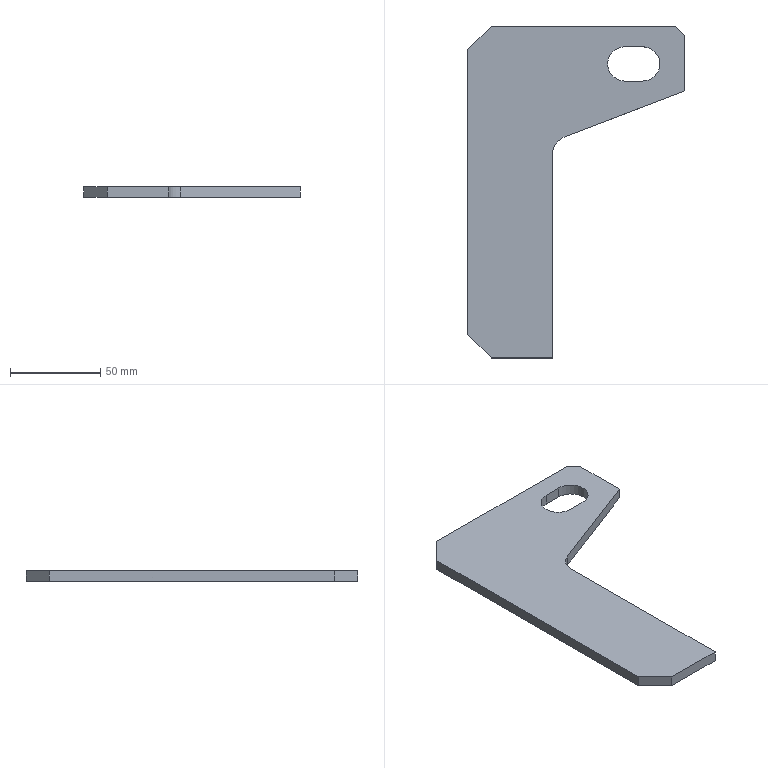Part | STEP file | 筋Plate-200×100-5 | 1 solid | 17 faces | box 120 x 184 x 6 mm | volume 69909 mm3 | plane 13 | cylinder 4 | commonest cylinder face diameters 19 x3 20 x1
STEP:
#1=CARTESIAN_POINT('',(0.,0.,0.));
#2=DIRECTION('',(0.,0.,1.));
#3=DIRECTION('',(1.,0.,0.));
#4=AXIS2_PLACEMENT_3D('',#1,#2,#3);
#5=CARTESIAN_POINT('',(27.,80.5,3.));
#6=VERTEX_POINT('',#5);
#7=CARTESIAN_POINT('',(27.,80.5,-3.));
#8=VERTEX_POINT('',#7);
#9=CARTESIAN_POINT('',(27.,80.5,-3.));
#10=DIRECTION('',(0.,0.,-1.));
#11=VECTOR('',#10,1.);
#12=LINE('',#9,#11);
#13=CARTESIAN_POINT('',(27.,71.,-3.));
#14=DIRECTION('',(0.,0.,-1.));
#15=DIRECTION('',(-1.,0.,0.));
#16=AXIS2_PLACEMENT_3D('',#13,#14,#15);
#17=CYLINDRICAL_SURFACE('',#16,9.5);
#18=CARTESIAN_POINT('',(1.571,0.));
#19=DIRECTION('',(0.,1.));
#20=VECTOR('',#19,1.);
#21=LINE('',#18,#20);
#22=(GEOMETRIC_REPRESENTATION_CONTEXT(2)PARAMETRIC_REPRESENTATION_CONTEXT()REPRESENTATION_CONTEXT('',''));
#23=DEFINITIONAL_REPRESENTATION('',(#21),#22);
#24=PCURVE('',#17,#23);
#25=CARTESIAN_POINT('',(37.,80.5,-3.));
#26=DIRECTION('',(0.,1.,0.));
#27=DIRECTION('',(0.,0.,1.));
#28=AXIS2_PLACEMENT_3D('',#25,#26,#27);
#29=PLANE('',#28);
#30=CARTESIAN_POINT('',(0.,-10.));
#31=DIRECTION('',(-1.,0.));
#32=VECTOR('',#31,1.);
#33=LINE('',#30,#32);
#34=(GEOMETRIC_REPRESENTATION_CONTEXT(2)PARAMETRIC_REPRESENTATION_CONTEXT()REPRESENTATION_CONTEXT('',''));
#35=DEFINITIONAL_REPRESENTATION('',(#33),#34);
#36=PCURVE('',#29,#35);
#37=SURFACE_CURVE('',#12,(#24,#36),.PCURVE_S1.);
#38=EDGE_CURVE('',#6,#8,#37,.T.);
#39=ORIENTED_EDGE('',*,*,#38,.T.);
#40=CARTESIAN_POINT('',(17.5,71.,-3.));
#41=VERTEX_POINT('',#40);
#42=CARTESIAN_POINT('',(27.,71.,-3.));
#43=DIRECTION('',(0.,0.,-1.));
#44=DIRECTION('',(-1.,0.,0.));
#45=AXIS2_PLACEMENT_3D('',#42,#43,#44);
#46=CIRCLE('',#45,9.5);
#47=CARTESIAN_POINT('',(0.,0.));
#48=DIRECTION('',(1.,0.));
#49=VECTOR('',#48,1.);
#50=LINE('',#47,#49);
#51=(GEOMETRIC_REPRESENTATION_CONTEXT(2)PARAMETRIC_REPRESENTATION_CONTEXT()REPRESENTATION_CONTEXT('',''));
#52=DEFINITIONAL_REPRESENTATION('',(#50),#51);
#53=PCURVE('',#17,#52);
#54=CARTESIAN_POINT('',(0.,0.,-3.));
#55=DIRECTION('',(0.,0.,1.));
#56=DIRECTION('',(1.,0.,0.));
#57=AXIS2_PLACEMENT_3D('',#54,#55,#56);
#58=PLANE('',#57);
#59=CARTESIAN_POINT('',(17.5,71.));
#60=CARTESIAN_POINT('',(17.5,87.454));
#61=CARTESIAN_POINT('',(31.75,79.227));
#62=CARTESIAN_POINT('',(46.,71.));
#63=CARTESIAN_POINT('',(31.75,62.773));
#64=CARTESIAN_POINT('',(17.5,54.546));
#65=CARTESIAN_POINT('',(17.5,71.));
#66=(BOUNDED_CURVE()B_SPLINE_CURVE(2,(#59,#60,#61,#62,#63,#64,#65),.UNSPECIFIED.,.T.,.F.)B_SPLINE_CURVE_WITH_KNOTS((1,2,2,2,2,1),(-2.094,0.,2.094,4.189,6.283,8.378),.UNSPECIFIED.)CURVE()GEOMETRIC_REPRESENTATION_ITEM()RATIONAL_B_SPLINE_CURVE((1.,0.5,1.,0.5,1.,0.5,1.))REPRESENTATION_ITEM(''));
#67=(GEOMETRIC_REPRESENTATION_CONTEXT(2)PARAMETRIC_REPRESENTATION_CONTEXT()REPRESENTATION_CONTEXT('',''));
#68=DEFINITIONAL_REPRESENTATION('',(#66),#67);
#69=PCURVE('',#58,#68);
#70=SURFACE_CURVE('',#46,(#53,#69),.PCURVE_S1.);
#71=EDGE_CURVE('',#41,#8,#70,.T.);
#72=ORIENTED_EDGE('',*,*,#71,.F.);
#73=CARTESIAN_POINT('',(17.5,71.,3.));
#74=VERTEX_POINT('',#73);
#75=CARTESIAN_POINT('',(17.5,71.,-3.));
#76=DIRECTION('',(0.,0.,-1.));
#77=VECTOR('',#76,1.);
#78=LINE('',#75,#77);
#79=CARTESIAN_POINT('',(0.,0.));
#80=DIRECTION('',(0.,1.));
#81=VECTOR('',#80,1.);
#82=LINE('',#79,#81);
#83=(GEOMETRIC_REPRESENTATION_CONTEXT(2)PARAMETRIC_REPRESENTATION_CONTEXT()REPRESENTATION_CONTEXT('',''));
#84=DEFINITIONAL_REPRESENTATION('',(#82),#83);
#85=PCURVE('',#17,#84);
#86=CARTESIAN_POINT('',(27.,71.,-3.));
#87=DIRECTION('',(0.,0.,-1.));
#88=DIRECTION('',(-1.,0.,0.));
#89=AXIS2_PLACEMENT_3D('',#86,#87,#88);
#90=CYLINDRICAL_SURFACE('',#89,9.5);
#91=CARTESIAN_POINT('',(6.283,0.));
#92=DIRECTION('',(0.,1.));
#93=VECTOR('',#92,1.);
#94=LINE('',#91,#93);
#95=(GEOMETRIC_REPRESENTATION_CONTEXT(2)PARAMETRIC_REPRESENTATION_CONTEXT()REPRESENTATION_CONTEXT('',''));
#96=DEFINITIONAL_REPRESENTATION('',(#94),#95);
#97=PCURVE('',#90,#96);
#98=SURFACE_CURVE('',#78,(#85,#97),.PCURVE_S1.);
#99=EDGE_CURVE('',#74,#41,#98,.T.);
#100=ORIENTED_EDGE('',*,*,#99,.F.);
#101=CARTESIAN_POINT('',(27.,71.,3.));
#102=DIRECTION('',(0.,0.,1.));
#103=DIRECTION('',(1.,0.,0.));
#104=AXIS2_PLACEMENT_3D('',#101,#102,#103);
#105=CIRCLE('',#104,9.5);
#106=CARTESIAN_POINT('',(3.142,-6.));
#107=DIRECTION('',(-1.,0.));
#108=VECTOR('',#107,1.);
#109=LINE('',#106,#108);
#110=(GEOMETRIC_REPRESENTATION_CONTEXT(2)PARAMETRIC_REPRESENTATION_CONTEXT()REPRESENTATION_CONTEXT('',''));
#111=DEFINITIONAL_REPRESENTATION('',(#109),#110);
#112=PCURVE('',#17,#111);
#113=CARTESIAN_POINT('',(0.,0.,3.));
#114=DIRECTION('',(0.,0.,1.));
#115=DIRECTION('',(1.,0.,0.));
#116=AXIS2_PLACEMENT_3D('',#113,#114,#115);
#117=PLANE('',#116);
#118=CARTESIAN_POINT('',(27.,71.));
#119=DIRECTION('',(1.,0.));
#120=AXIS2_PLACEMENT_2D('',#118,#119);
#121=CIRCLE('',#120,9.5);
#122=(GEOMETRIC_REPRESENTATION_CONTEXT(2)PARAMETRIC_REPRESENTATION_CONTEXT()REPRESENTATION_CONTEXT('',''));
#123=DEFINITIONAL_REPRESENTATION('',(#121),#122);
#124=PCURVE('',#117,#123);
#125=SURFACE_CURVE('',#105,(#112,#124),.PCURVE_S1.);
#126=EDGE_CURVE('',#6,#74,#125,.T.);
#127=ORIENTED_EDGE('',*,*,#126,.F.);
#128=EDGE_LOOP('',(#39,#72,#100,#127));
#129=FACE_BOUND('',#128,.F.);
#130=ADVANCED_FACE('',(#129),#17,.F.);
#131=CARTESIAN_POINT('',(60.,56.,-3.));
#132=VERTEX_POINT('',#131);
#133=CARTESIAN_POINT('',(60.,87.,-3.));
#134=VERTEX_POINT('',#133);
#135=CARTESIAN_POINT('',(60.,92.,-3.));
#136=DIRECTION('',(0.,1.,0.));
#137=VECTOR('',#136,1.);
#138=LINE('',#135,#137);
#139=CARTESIAN_POINT('',(60.,92.,3.));
#140=DIRECTION('',(-1.,0.,0.));
#141=DIRECTION('',(0.,-1.,0.));
#142=AXIS2_PLACEMENT_3D('',#139,#140,#141);
#143=PLANE('',#142);
#144=CARTESIAN_POINT('',(0.,-6.));
#145=DIRECTION('',(-1.,0.));
#146=VECTOR('',#145,1.);
#147=LINE('',#144,#146);
#148=(GEOMETRIC_REPRESENTATION_CONTEXT(2)PARAMETRIC_REPRESENTATION_CONTEXT()REPRESENTATION_CONTEXT('',''));
#149=DEFINITIONAL_REPRESENTATION('',(#147),#148);
#150=PCURVE('',#143,#149);
#151=CARTESIAN_POINT('',(60.,92.));
#152=DIRECTION('',(0.,1.));
#153=VECTOR('',#152,1.);
#154=LINE('',#151,#153);
#155=(GEOMETRIC_REPRESENTATION_CONTEXT(2)PARAMETRIC_REPRESENTATION_CONTEXT()REPRESENTATION_CONTEXT('',''));
#156=DEFINITIONAL_REPRESENTATION('',(#154),#155);
#157=PCURVE('',#58,#156);
#158=SURFACE_CURVE('',#138,(#150,#157),.PCURVE_S1.);
#159=EDGE_CURVE('',#132,#134,#158,.T.);
#160=ORIENTED_EDGE('',*,*,#159,.T.);
#161=CARTESIAN_POINT('',(60.,87.,3.));
#162=VERTEX_POINT('',#161);
#163=CARTESIAN_POINT('',(60.,87.,3.));
#164=DIRECTION('',(0.,0.,1.));
#165=VECTOR('',#164,1.);
#166=LINE('',#163,#165);
#167=CARTESIAN_POINT('',(5.,0.));
#168=DIRECTION('',(0.,1.));
#169=VECTOR('',#168,1.);
#170=LINE('',#167,#169);
#171=(GEOMETRIC_REPRESENTATION_CONTEXT(2)PARAMETRIC_REPRESENTATION_CONTEXT()REPRESENTATION_CONTEXT('',''));
#172=DEFINITIONAL_REPRESENTATION('',(#170),#171);
#173=PCURVE('',#143,#172);
#174=CARTESIAN_POINT('',(55.,92.,3.));
#175=DIRECTION('',(-0.7071,-0.7071,0.));
#176=DIRECTION('',(0.,0.,-1.));
#177=AXIS2_PLACEMENT_3D('',#174,#175,#176);
#178=PLANE('',#177);
#179=CARTESIAN_POINT('',(0.,7.071));
#180=DIRECTION('',(-1.,0.));
#181=VECTOR('',#180,1.);
#182=LINE('',#179,#181);
#183=(GEOMETRIC_REPRESENTATION_CONTEXT(2)PARAMETRIC_REPRESENTATION_CONTEXT()REPRESENTATION_CONTEXT('',''));
#184=DEFINITIONAL_REPRESENTATION('',(#182),#183);
#185=PCURVE('',#178,#184);
#186=SURFACE_CURVE('',#166,(#173,#185),.PCURVE_S1.);
#187=EDGE_CURVE('',#134,#162,#186,.T.);
#188=ORIENTED_EDGE('',*,*,#187,.T.);
#189=CARTESIAN_POINT('',(60.,56.,3.));
#190=VERTEX_POINT('',#189);
#191=CARTESIAN_POINT('',(60.,92.,3.));
#192=DIRECTION('',(0.,1.,0.));
#193=VECTOR('',#192,1.);
#194=LINE('',#191,#193);
#195=CARTESIAN_POINT('',(0.,0.));
#196=DIRECTION('',(-1.,0.));
#197=VECTOR('',#196,1.);
#198=LINE('',#195,#197);
#199=(GEOMETRIC_REPRESENTATION_CONTEXT(2)PARAMETRIC_REPRESENTATION_CONTEXT()REPRESENTATION_CONTEXT('',''));
#200=DEFINITIONAL_REPRESENTATION('',(#198),#199);
#201=PCURVE('',#143,#200);
#202=CARTESIAN_POINT('',(60.,92.));
#203=DIRECTION('',(0.,1.));
#204=VECTOR('',#203,1.);
#205=LINE('',#202,#204);
#206=(GEOMETRIC_REPRESENTATION_CONTEXT(2)PARAMETRIC_REPRESENTATION_CONTEXT()REPRESENTATION_CONTEXT('',''));
#207=DEFINITIONAL_REPRESENTATION('',(#205),#206);
#208=PCURVE('',#117,#207);
#209=SURFACE_CURVE('',#194,(#201,#208),.PCURVE_S1.);
#210=EDGE_CURVE('',#190,#162,#209,.T.);
#211=ORIENTED_EDGE('',*,*,#210,.F.);
#212=CARTESIAN_POINT('',(60.,56.,-3.));
#213=DIRECTION('',(0.,0.,1.));
#214=VECTOR('',#213,1.);
#215=LINE('',#212,#214);
#216=CARTESIAN_POINT('',(36.,-6.));
#217=DIRECTION('',(0.,1.));
#218=VECTOR('',#217,1.);
#219=LINE('',#216,#218);
#220=(GEOMETRIC_REPRESENTATION_CONTEXT(2)PARAMETRIC_REPRESENTATION_CONTEXT()REPRESENTATION_CONTEXT('',''));
#221=DEFINITIONAL_REPRESENTATION('',(#219),#220);
#222=PCURVE('',#143,#221);
#223=CARTESIAN_POINT('',(60.,56.,-3.));
#224=DIRECTION('',(-0.3581,0.9337,0.));
#225=DIRECTION('',(-0.9337,-0.3581,0.));
#226=AXIS2_PLACEMENT_3D('',#223,#224,#225);
#227=PLANE('',#226);
#228=CARTESIAN_POINT('',(0.,0.));
#229=DIRECTION('',(0.,1.));
#230=VECTOR('',#229,1.);
#231=LINE('',#228,#230);
#232=(GEOMETRIC_REPRESENTATION_CONTEXT(2)PARAMETRIC_REPRESENTATION_CONTEXT()REPRESENTATION_CONTEXT('',''));
#233=DEFINITIONAL_REPRESENTATION('',(#231),#232);
#234=PCURVE('',#227,#233);
#235=SURFACE_CURVE('',#215,(#222,#234),.PCURVE_S1.);
#236=EDGE_CURVE('',#132,#190,#235,.T.);
#237=ORIENTED_EDGE('',*,*,#236,.F.);
#238=EDGE_LOOP('',(#160,#188,#211,#237));
#239=FACE_BOUND('',#238,.T.);
#240=ADVANCED_FACE('',(#239),#143,.F.);
#241=CARTESIAN_POINT('',(55.,92.,3.));
#242=VERTEX_POINT('',#241);
#243=CARTESIAN_POINT('',(-47.,92.,3.));
#244=VERTEX_POINT('',#243);
#245=CARTESIAN_POINT('',(-60.,92.,3.));
#246=DIRECTION('',(-1.,0.,0.));
#247=VECTOR('',#246,1.);
#248=LINE('',#245,#247);
#249=CARTESIAN_POINT('',(-60.,92.,3.));
#250=DIRECTION('',(0.,-1.,0.));
#251=DIRECTION('',(0.,0.,-1.));
#252=AXIS2_PLACEMENT_3D('',#249,#250,#251);
#253=PLANE('',#252);
#254=CARTESIAN_POINT('',(0.,0.));
#255=DIRECTION('',(0.,-1.));
#256=VECTOR('',#255,1.);
#257=LINE('',#254,#256);
#258=(GEOMETRIC_REPRESENTATION_CONTEXT(2)PARAMETRIC_REPRESENTATION_CONTEXT()REPRESENTATION_CONTEXT('',''));
#259=DEFINITIONAL_REPRESENTATION('',(#257),#258);
#260=PCURVE('',#253,#259);
#261=CARTESIAN_POINT('',(-60.,92.));
#262=DIRECTION('',(-1.,0.));
#263=VECTOR('',#262,1.);
#264=LINE('',#261,#263);
#265=(GEOMETRIC_REPRESENTATION_CONTEXT(2)PARAMETRIC_REPRESENTATION_CONTEXT()REPRESENTATION_CONTEXT('',''));
#266=DEFINITIONAL_REPRESENTATION('',(#264),#265);
#267=PCURVE('',#117,#266);
#268=SURFACE_CURVE('',#248,(#260,#267),.PCURVE_S1.);
#269=EDGE_CURVE('',#242,#244,#268,.T.);
#270=ORIENTED_EDGE('',*,*,#269,.F.);
#271=CARTESIAN_POINT('',(55.,92.,-3.));
#272=VERTEX_POINT('',#271);
#273=CARTESIAN_POINT('',(55.,92.,3.));
#274=DIRECTION('',(0.,0.,-1.));
#275=VECTOR('',#274,1.);
#276=LINE('',#273,#275);
#277=CARTESIAN_POINT('',(0.,115.));
#278=DIRECTION('',(1.,0.));
#279=VECTOR('',#278,1.);
#280=LINE('',#277,#279);
#281=(GEOMETRIC_REPRESENTATION_CONTEXT(2)PARAMETRIC_REPRESENTATION_CONTEXT()REPRESENTATION_CONTEXT('',''));
#282=DEFINITIONAL_REPRESENTATION('',(#280),#281);
#283=PCURVE('',#253,#282);
#284=CARTESIAN_POINT('',(0.,0.));
#285=DIRECTION('',(1.,0.));
#286=VECTOR('',#285,1.);
#287=LINE('',#284,#286);
#288=(GEOMETRIC_REPRESENTATION_CONTEXT(2)PARAMETRIC_REPRESENTATION_CONTEXT()REPRESENTATION_CONTEXT('',''));
#289=DEFINITIONAL_REPRESENTATION('',(#287),#288);
#290=PCURVE('',#178,#289);
#291=SURFACE_CURVE('',#276,(#283,#290),.PCURVE_S1.);
#292=EDGE_CURVE('',#242,#272,#291,.T.);
#293=ORIENTED_EDGE('',*,*,#292,.T.);
#294=CARTESIAN_POINT('',(-47.,92.,-3.));
#295=VERTEX_POINT('',#294);
#296=CARTESIAN_POINT('',(-60.,92.,-3.));
#297=DIRECTION('',(-1.,0.,0.));
#298=VECTOR('',#297,1.);
#299=LINE('',#296,#298);
#300=CARTESIAN_POINT('',(6.,0.));
#301=DIRECTION('',(0.,-1.));
#302=VECTOR('',#301,1.);
#303=LINE('',#300,#302);
#304=(GEOMETRIC_REPRESENTATION_CONTEXT(2)PARAMETRIC_REPRESENTATION_CONTEXT()REPRESENTATION_CONTEXT('',''));
#305=DEFINITIONAL_REPRESENTATION('',(#303),#304);
#306=PCURVE('',#253,#305);
#307=CARTESIAN_POINT('',(-60.,92.));
#308=DIRECTION('',(-1.,0.));
#309=VECTOR('',#308,1.);
#310=LINE('',#307,#309);
#311=(GEOMETRIC_REPRESENTATION_CONTEXT(2)PARAMETRIC_REPRESENTATION_CONTEXT()REPRESENTATION_CONTEXT('',''));
#312=DEFINITIONAL_REPRESENTATION('',(#310),#311);
#313=PCURVE('',#58,#312);
#314=SURFACE_CURVE('',#299,(#306,#313),.PCURVE_S1.);
#315=EDGE_CURVE('',#272,#295,#314,.T.);
#316=ORIENTED_EDGE('',*,*,#315,.T.);
#317=CARTESIAN_POINT('',(-47.,92.,3.));
#318=DIRECTION('',(0.,0.,1.));
#319=VECTOR('',#318,1.);
#320=LINE('',#317,#319);
#321=CARTESIAN_POINT('',(0.,13.));
#322=DIRECTION('',(-1.,0.));
#323=VECTOR('',#322,1.);
#324=LINE('',#321,#323);
#325=(GEOMETRIC_REPRESENTATION_CONTEXT(2)PARAMETRIC_REPRESENTATION_CONTEXT()REPRESENTATION_CONTEXT('',''));
#326=DEFINITIONAL_REPRESENTATION('',(#324),#325);
#327=PCURVE('',#253,#326);
#328=CARTESIAN_POINT('',(-60.,79.,3.));
#329=DIRECTION('',(0.7071,-0.7071,0.));
#330=DIRECTION('',(0.,0.,-1.));
#331=AXIS2_PLACEMENT_3D('',#328,#329,#330);
#332=PLANE('',#331);
#333=CARTESIAN_POINT('',(0.,18.385));
#334=DIRECTION('',(-1.,0.));
#335=VECTOR('',#334,1.);
#336=LINE('',#333,#335);
#337=(GEOMETRIC_REPRESENTATION_CONTEXT(2)PARAMETRIC_REPRESENTATION_CONTEXT()REPRESENTATION_CONTEXT('',''));
#338=DEFINITIONAL_REPRESENTATION('',(#336),#337);
#339=PCURVE('',#332,#338);
#340=SURFACE_CURVE('',#320,(#327,#339),.PCURVE_S1.);
#341=EDGE_CURVE('',#295,#244,#340,.T.);
#342=ORIENTED_EDGE('',*,*,#341,.T.);
#343=EDGE_LOOP('',(#270,#293,#316,#342));
#344=FACE_BOUND('',#343,.T.);
#345=ADVANCED_FACE('',(#344),#253,.F.);
#346=CARTESIAN_POINT('',(-60.,79.,-3.));
#347=VERTEX_POINT('',#346);
#348=CARTESIAN_POINT('',(-60.,-79.,-3.));
#349=VERTEX_POINT('',#348);
#350=CARTESIAN_POINT('',(-60.,92.,-3.));
#351=DIRECTION('',(0.,-1.,0.));
#352=VECTOR('',#351,1.);
#353=LINE('',#350,#352);
#354=CARTESIAN_POINT('',(-60.,92.,3.));
#355=DIRECTION('',(1.,0.,0.));
#356=DIRECTION('',(0.,1.,0.));
#357=AXIS2_PLACEMENT_3D('',#354,#355,#356);
#358=PLANE('',#357);
#359=CARTESIAN_POINT('',(0.,-6.));
#360=DIRECTION('',(-1.,0.));
#361=VECTOR('',#360,1.);
#362=LINE('',#359,#361);
#363=(GEOMETRIC_REPRESENTATION_CONTEXT(2)PARAMETRIC_REPRESENTATION_CONTEXT()REPRESENTATION_CONTEXT('',''));
#364=DEFINITIONAL_REPRESENTATION('',(#362),#363);
#365=PCURVE('',#358,#364);
#366=CARTESIAN_POINT('',(-60.,92.));
#367=DIRECTION('',(0.,-1.));
#368=VECTOR('',#367,1.);
#369=LINE('',#366,#368);
#370=(GEOMETRIC_REPRESENTATION_CONTEXT(2)PARAMETRIC_REPRESENTATION_CONTEXT()REPRESENTATION_CONTEXT('',''));
#371=DEFINITIONAL_REPRESENTATION('',(#369),#370);
#372=PCURVE('',#58,#371);
#373=SURFACE_CURVE('',#353,(#365,#372),.PCURVE_S1.);
#374=EDGE_CURVE('',#347,#349,#373,.T.);
#375=ORIENTED_EDGE('',*,*,#374,.T.);
#376=CARTESIAN_POINT('',(-60.,-79.,3.));
#377=VERTEX_POINT('',#376);
#378=CARTESIAN_POINT('',(-60.,-79.,3.));
#379=DIRECTION('',(0.,0.,1.));
#380=VECTOR('',#379,1.);
#381=LINE('',#378,#380);
#382=CARTESIAN_POINT('',(-171.,0.));
#383=DIRECTION('',(0.,1.));
#384=VECTOR('',#383,1.);
#385=LINE('',#382,#384);
#386=(GEOMETRIC_REPRESENTATION_CONTEXT(2)PARAMETRIC_REPRESENTATION_CONTEXT()REPRESENTATION_CONTEXT('',''));
#387=DEFINITIONAL_REPRESENTATION('',(#385),#386);
#388=PCURVE('',#358,#387);
#389=CARTESIAN_POINT('',(-47.,-92.,3.));
#390=DIRECTION('',(0.7071,0.7071,0.));
#391=DIRECTION('',(0.,0.,-1.));
#392=AXIS2_PLACEMENT_3D('',#389,#390,#391);
#393=PLANE('',#392);
#394=CARTESIAN_POINT('',(0.,18.385));
#395=DIRECTION('',(-1.,0.));
#396=VECTOR('',#395,1.);
#397=LINE('',#394,#396);
#398=(GEOMETRIC_REPRESENTATION_CONTEXT(2)PARAMETRIC_REPRESENTATION_CONTEXT()REPRESENTATION_CONTEXT('',''));
#399=DEFINITIONAL_REPRESENTATION('',(#397),#398);
#400=PCURVE('',#393,#399);
#401=SURFACE_CURVE('',#381,(#388,#400),.PCURVE_S1.);
#402=EDGE_CURVE('',#349,#377,#401,.T.);
#403=ORIENTED_EDGE('',*,*,#402,.T.);
#404=CARTESIAN_POINT('',(-60.,79.,3.));
#405=VERTEX_POINT('',#404);
#406=CARTESIAN_POINT('',(-60.,92.,3.));
#407=DIRECTION('',(0.,-1.,0.));
#408=VECTOR('',#407,1.);
#409=LINE('',#406,#408);
#410=CARTESIAN_POINT('',(0.,0.));
#411=DIRECTION('',(-1.,0.));
#412=VECTOR('',#411,1.);
#413=LINE('',#410,#412);
#414=(GEOMETRIC_REPRESENTATION_CONTEXT(2)PARAMETRIC_REPRESENTATION_CONTEXT()REPRESENTATION_CONTEXT('',''));
#415=DEFINITIONAL_REPRESENTATION('',(#413),#414);
#416=PCURVE('',#358,#415);
#417=CARTESIAN_POINT('',(-60.,92.));
#418=DIRECTION('',(0.,-1.));
#419=VECTOR('',#418,1.);
#420=LINE('',#417,#419);
#421=(GEOMETRIC_REPRESENTATION_CONTEXT(2)PARAMETRIC_REPRESENTATION_CONTEXT()REPRESENTATION_CONTEXT('',''));
#422=DEFINITIONAL_REPRESENTATION('',(#420),#421);
#423=PCURVE('',#117,#422);
#424=SURFACE_CURVE('',#409,(#416,#423),.PCURVE_S1.);
#425=EDGE_CURVE('',#405,#377,#424,.T.);
#426=ORIENTED_EDGE('',*,*,#425,.F.);
#427=CARTESIAN_POINT('',(-60.,79.,3.));
#428=DIRECTION('',(0.,0.,-1.));
#429=VECTOR('',#428,1.);
#430=LINE('',#427,#429);
#431=CARTESIAN_POINT('',(-13.,0.));
#432=DIRECTION('',(0.,-1.));
#433=VECTOR('',#432,1.);
#434=LINE('',#431,#433);
#435=(GEOMETRIC_REPRESENTATION_CONTEXT(2)PARAMETRIC_REPRESENTATION_CONTEXT()REPRESENTATION_CONTEXT('',''));
#436=DEFINITIONAL_REPRESENTATION('',(#434),#435);
#437=PCURVE('',#358,#436);
#438=CARTESIAN_POINT('',(0.,0.));
#439=DIRECTION('',(1.,0.));
#440=VECTOR('',#439,1.);
#441=LINE('',#438,#440);
#442=(GEOMETRIC_REPRESENTATION_CONTEXT(2)PARAMETRIC_REPRESENTATION_CONTEXT()REPRESENTATION_CONTEXT('',''));
#443=DEFINITIONAL_REPRESENTATION('',(#441),#442);
#444=PCURVE('',#332,#443);
#445=SURFACE_CURVE('',#430,(#437,#444),.PCURVE_S1.);
#446=EDGE_CURVE('',#405,#347,#445,.T.);
#447=ORIENTED_EDGE('',*,*,#446,.T.);
#448=EDGE_LOOP('',(#375,#403,#426,#447));
#449=FACE_BOUND('',#448,.T.);
#450=ADVANCED_FACE('',(#449),#358,.F.);
#451=CARTESIAN_POINT('',(-47.,-92.,3.));
#452=VERTEX_POINT('',#451);
#453=CARTESIAN_POINT('',(-13.,-92.,3.));
#454=VERTEX_POINT('',#453);
#455=CARTESIAN_POINT('',(-60.,-92.,3.));
#456=DIRECTION('',(1.,0.,0.));
#457=VECTOR('',#456,1.);
#458=LINE('',#455,#457);
#459=CARTESIAN_POINT('',(-60.,-92.,3.));
#460=DIRECTION('',(0.,1.,0.));
#461=DIRECTION('',(0.,0.,1.));
#462=AXIS2_PLACEMENT_3D('',#459,#460,#461);
#463=PLANE('',#462);
#464=CARTESIAN_POINT('',(0.,0.));
#465=DIRECTION('',(0.,1.));
#466=VECTOR('',#465,1.);
#467=LINE('',#464,#466);
#468=(GEOMETRIC_REPRESENTATION_CONTEXT(2)PARAMETRIC_REPRESENTATION_CONTEXT()REPRESENTATION_CONTEXT('',''));
#469=DEFINITIONAL_REPRESENTATION('',(#467),#468);
#470=PCURVE('',#463,#469);
#471=CARTESIAN_POINT('',(-60.,-92.));
#472=DIRECTION('',(1.,0.));
#473=VECTOR('',#472,1.);
#474=LINE('',#471,#473);
#475=(GEOMETRIC_REPRESENTATION_CONTEXT(2)PARAMETRIC_REPRESENTATION_CONTEXT()REPRESENTATION_CONTEXT('',''));
#476=DEFINITIONAL_REPRESENTATION('',(#474),#475);
#477=PCURVE('',#117,#476);
#478=SURFACE_CURVE('',#458,(#470,#477),.PCURVE_S1.);
#479=EDGE_CURVE('',#452,#454,#478,.T.);
#480=ORIENTED_EDGE('',*,*,#479,.F.);
#481=CARTESIAN_POINT('',(-47.,-92.,-3.));
#482=VERTEX_POINT('',#481);
#483=CARTESIAN_POINT('',(-47.,-92.,3.));
#484=DIRECTION('',(0.,0.,-1.));
#485=VECTOR('',#484,1.);
#486=LINE('',#483,#485);
#487=CARTESIAN_POINT('',(0.,13.));
#488=DIRECTION('',(-1.,0.));
#489=VECTOR('',#488,1.);
#490=LINE('',#487,#489);
#491=(GEOMETRIC_REPRESENTATION_CONTEXT(2)PARAMETRIC_REPRESENTATION_CONTEXT()REPRESENTATION_CONTEXT('',''));
#492=DEFINITIONAL_REPRESENTATION('',(#490),#491);
#493=PCURVE('',#463,#492);
#494=CARTESIAN_POINT('',(0.,0.));
#495=DIRECTION('',(1.,0.));
#496=VECTOR('',#495,1.);
#497=LINE('',#494,#496);
#498=(GEOMETRIC_REPRESENTATION_CONTEXT(2)PARAMETRIC_REPRESENTATION_CONTEXT()REPRESENTATION_CONTEXT('',''));
#499=DEFINITIONAL_REPRESENTATION('',(#497),#498);
#500=PCURVE('',#393,#499);
#501=SURFACE_CURVE('',#486,(#493,#500),.PCURVE_S1.);
#502=EDGE_CURVE('',#452,#482,#501,.T.);
#503=ORIENTED_EDGE('',*,*,#502,.T.);
#504=CARTESIAN_POINT('',(-13.,-92.,-3.));
#505=VERTEX_POINT('',#504);
#506=CARTESIAN_POINT('',(-60.,-92.,-3.));
#507=DIRECTION('',(1.,0.,0.));
#508=VECTOR('',#507,1.);
#509=LINE('',#506,#508);
#510=CARTESIAN_POINT('',(-6.,0.));
#511=DIRECTION('',(0.,1.));
#512=VECTOR('',#511,1.);
#513=LINE('',#510,#512);
#514=(GEOMETRIC_REPRESENTATION_CONTEXT(2)PARAMETRIC_REPRESENTATION_CONTEXT()REPRESENTATION_CONTEXT('',''));
#515=DEFINITIONAL_REPRESENTATION('',(#513),#514);
#516=PCURVE('',#463,#515);
#517=CARTESIAN_POINT('',(-60.,-92.));
#518=DIRECTION('',(1.,0.));
#519=VECTOR('',#518,1.);
#520=LINE('',#517,#519);
#521=(GEOMETRIC_REPRESENTATION_CONTEXT(2)PARAMETRIC_REPRESENTATION_CONTEXT()REPRESENTATION_CONTEXT('',''));
#522=DEFINITIONAL_REPRESENTATION('',(#520),#521);
#523=PCURVE('',#58,#522);
#524=SURFACE_CURVE('',#509,(#516,#523),.PCURVE_S1.);
#525=EDGE_CURVE('',#482,#505,#524,.T.);
#526=ORIENTED_EDGE('',*,*,#525,.T.);
#527=CARTESIAN_POINT('',(-13.,-92.,-3.));
#528=DIRECTION('',(0.,0.,1.));
#529=VECTOR('',#528,1.);
#530=LINE('',#527,#529);
#531=CARTESIAN_POINT('',(-6.,47.));
#532=DIRECTION('',(1.,0.));
#533=VECTOR('',#532,1.);
#534=LINE('',#531,#533);
#535=(GEOMETRIC_REPRESENTATION_CONTEXT(2)PARAMETRIC_REPRESENTATION_CONTEXT()REPRESENTATION_CONTEXT('',''));
#536=DEFINITIONAL_REPRESENTATION('',(#534),#535);
#537=PCURVE('',#463,#536);
#538=CARTESIAN_POINT('',(-13.,-92.,-3.));
#539=DIRECTION('',(-1.,0.,0.));
#540=DIRECTION('',(0.,-1.,0.));
#541=AXIS2_PLACEMENT_3D('',#538,#539,#540);
#542=PLANE('',#541);
#543=CARTESIAN_POINT('',(0.,0.));
#544=DIRECTION('',(0.,1.));
#545=VECTOR('',#544,1.);
#546=LINE('',#543,#545);
#547=(GEOMETRIC_REPRESENTATION_CONTEXT(2)PARAMETRIC_REPRESENTATION_CONTEXT()REPRESENTATION_CONTEXT('',''));
#548=DEFINITIONAL_REPRESENTATION('',(#546),#547);
#549=PCURVE('',#542,#548);
#550=SURFACE_CURVE('',#530,(#537,#549),.PCURVE_S1.);
#551=EDGE_CURVE('',#505,#454,#550,.T.);
#552=ORIENTED_EDGE('',*,*,#551,.T.);
#553=EDGE_LOOP('',(#480,#503,#526,#552));
#554=FACE_BOUND('',#553,.T.);
#555=ADVANCED_FACE('',(#554),#463,.F.);
#556=CARTESIAN_POINT('',(37.,61.5,3.));
#557=VERTEX_POINT('',#556);
#558=CARTESIAN_POINT('',(37.,80.5,3.));
#559=VERTEX_POINT('',#558);
#560=CARTESIAN_POINT('',(37.,71.,3.));
#561=DIRECTION('',(0.,0.,1.));
#562=DIRECTION('',(1.,0.,0.));
#563=AXIS2_PLACEMENT_3D('',#560,#561,#562);
#564=CIRCLE('',#563,9.5);
#565=CARTESIAN_POINT('',(37.,71.));
#566=DIRECTION('',(1.,0.));
#567=AXIS2_PLACEMENT_2D('',#565,#566);
#568=CIRCLE('',#567,9.5);
#569=(GEOMETRIC_REPRESENTATION_CONTEXT(2)PARAMETRIC_REPRESENTATION_CONTEXT()REPRESENTATION_CONTEXT('',''));
#570=DEFINITIONAL_REPRESENTATION('',(#568),#569);
#571=PCURVE('',#117,#570);
#572=CARTESIAN_POINT('',(37.,71.,-3.));
#573=DIRECTION('',(0.,0.,-1.));
#574=DIRECTION('',(-1.,0.,0.));
#575=AXIS2_PLACEMENT_3D('',#572,#573,#574);
#576=CYLINDRICAL_SURFACE('',#575,9.5);
#577=CARTESIAN_POINT('',(9.425,-6.));
#578=DIRECTION('',(-1.,0.));
#579=VECTOR('',#578,1.);
#580=LINE('',#577,#579);
#581=(GEOMETRIC_REPRESENTATION_CONTEXT(2)PARAMETRIC_REPRESENTATION_CONTEXT()REPRESENTATION_CONTEXT('',''));
#582=DEFINITIONAL_REPRESENTATION('',(#580),#581);
#583=PCURVE('',#576,#582);
#584=SURFACE_CURVE('',#564,(#571,#583),.PCURVE_S1.);
#585=EDGE_CURVE('',#557,#559,#584,.T.);
#586=ORIENTED_EDGE('',*,*,#585,.F.);
#587=CARTESIAN_POINT('',(27.,61.5,3.));
#588=VERTEX_POINT('',#587);
#589=CARTESIAN_POINT('',(0.,61.5,3.));
#590=DIRECTION('',(1.,0.,0.));
#591=VECTOR('',#590,1.);
#592=LINE('',#589,#591);
#593=CARTESIAN_POINT('',(0.,61.5));
#594=DIRECTION('',(1.,0.));
#595=VECTOR('',#594,1.);
#596=LINE('',#593,#595);
#597=(GEOMETRIC_REPRESENTATION_CONTEXT(2)PARAMETRIC_REPRESENTATION_CONTEXT()REPRESENTATION_CONTEXT('',''));
#598=DEFINITIONAL_REPRESENTATION('',(#596),#597);
#599=PCURVE('',#117,#598);
#600=CARTESIAN_POINT('',(37.,61.5,-3.));
#601=DIRECTION('',(0.,-1.,0.));
#602=DIRECTION('',(0.,0.,-1.));
#603=AXIS2_PLACEMENT_3D('',#600,#601,#602);
#604=PLANE('',#603);
#605=CARTESIAN_POINT('',(-6.,-37.));
#606=DIRECTION('',(0.,1.));
#607=VECTOR('',#606,1.);
#608=LINE('',#605,#607);
#609=(GEOMETRIC_REPRESENTATION_CONTEXT(2)PARAMETRIC_REPRESENTATION_CONTEXT()REPRESENTATION_CONTEXT('',''));
#610=DEFINITIONAL_REPRESENTATION('',(#608),#609);
#611=PCURVE('',#604,#610);
#612=SURFACE_CURVE('',#592,(#599,#611),.PCURVE_S1.);
#613=EDGE_CURVE('',#588,#557,#612,.T.);
#614=ORIENTED_EDGE('',*,*,#613,.F.);
#615=CARTESIAN_POINT('',(27.,71.,3.));
#616=DIRECTION('',(0.,0.,1.));
#617=DIRECTION('',(1.,0.,0.));
#618=AXIS2_PLACEMENT_3D('',#615,#616,#617);
#619=CIRCLE('',#618,9.5);
#620=CARTESIAN_POINT('',(27.,71.));
#621=DIRECTION('',(1.,0.));
#622=AXIS2_PLACEMENT_2D('',#620,#621);
#623=CIRCLE('',#622,9.5);
#624=(GEOMETRIC_REPRESENTATION_CONTEXT(2)PARAMETRIC_REPRESENTATION_CONTEXT()REPRESENTATION_CONTEXT('',''));
#625=DEFINITIONAL_REPRESENTATION('',(#623),#624);
#626=PCURVE('',#117,#625);
#627=CARTESIAN_POINT('',(9.425,-6.));
#628=DIRECTION('',(-1.,0.));
#629=VECTOR('',#628,1.);
#630=LINE('',#627,#629);
#631=(GEOMETRIC_REPRESENTATION_CONTEXT(2)PARAMETRIC_REPRESENTATION_CONTEXT()REPRESENTATION_CONTEXT('',''));
#632=DEFINITIONAL_REPRESENTATION('',(#630),#631);
#633=PCURVE('',#90,#632);
#634=SURFACE_CURVE('',#619,(#626,#633),.PCURVE_S1.);
#635=EDGE_CURVE('',#74,#588,#634,.T.);
#636=ORIENTED_EDGE('',*,*,#635,.F.);
#637=ORIENTED_EDGE('',*,*,#126,.F.);
#638=CARTESIAN_POINT('',(0.,80.5,3.));
#639=DIRECTION('',(-1.,0.,0.));
#640=VECTOR('',#639,1.);
#641=LINE('',#638,#640);
#642=CARTESIAN_POINT('',(0.,80.5));
#643=DIRECTION('',(-1.,0.));
#644=VECTOR('',#643,1.);
#645=LINE('',#642,#644);
#646=(GEOMETRIC_REPRESENTATION_CONTEXT(2)PARAMETRIC_REPRESENTATION_CONTEXT()REPRESENTATION_CONTEXT('',''));
#647=DEFINITIONAL_REPRESENTATION('',(#645),#646);
#648=PCURVE('',#117,#647);
#649=CARTESIAN_POINT('',(6.,-37.));
#650=DIRECTION('',(0.,-1.));
#651=VECTOR('',#650,1.);
#652=LINE('',#649,#651);
#653=(GEOMETRIC_REPRESENTATION_CONTEXT(2)PARAMETRIC_REPRESENTATION_CONTEXT()REPRESENTATION_CONTEXT('',''));
#654=DEFINITIONAL_REPRESENTATION('',(#652),#653);
#655=PCURVE('',#29,#654);
#656=SURFACE_CURVE('',#641,(#648,#655),.PCURVE_S1.);
#657=EDGE_CURVE('',#559,#6,#656,.T.);
#658=ORIENTED_EDGE('',*,*,#657,.F.);
#659=EDGE_LOOP('',(#586,#614,#636,#637,#658));
#660=FACE_BOUND('',#659,.T.);
#661=ORIENTED_EDGE('',*,*,#210,.T.);
#662=CARTESIAN_POINT('',(73.5,73.5,3.));
#663=DIRECTION('',(-0.7071,0.7071,0.));
#664=VECTOR('',#663,1.);
#665=LINE('',#662,#664);
#666=CARTESIAN_POINT('',(73.5,73.5));
#667=DIRECTION('',(-0.7071,0.7071));
#668=VECTOR('',#667,1.);
#669=LINE('',#666,#668);
#670=(GEOMETRIC_REPRESENTATION_CONTEXT(2)PARAMETRIC_REPRESENTATION_CONTEXT()REPRESENTATION_CONTEXT('',''));
#671=DEFINITIONAL_REPRESENTATION('',(#669),#670);
#672=PCURVE('',#117,#671);
#673=CARTESIAN_POINT('',(0.,26.163));
#674=DIRECTION('',(0.,-1.));
#675=VECTOR('',#674,1.);
#676=LINE('',#673,#675);
#677=(GEOMETRIC_REPRESENTATION_CONTEXT(2)PARAMETRIC_REPRESENTATION_CONTEXT()REPRESENTATION_CONTEXT('',''));
#678=DEFINITIONAL_REPRESENTATION('',(#676),#677);
#679=PCURVE('',#178,#678);
#680=SURFACE_CURVE('',#665,(#672,#679),.PCURVE_S1.);
#681=EDGE_CURVE('',#162,#242,#680,.T.);
#682=ORIENTED_EDGE('',*,*,#681,.T.);
#683=ORIENTED_EDGE('',*,*,#269,.T.);
#684=CARTESIAN_POINT('',(-69.5,69.5,3.));
#685=DIRECTION('',(-0.7071,-0.7071,0.));
#686=VECTOR('',#685,1.);
#687=LINE('',#684,#686);
#688=CARTESIAN_POINT('',(-69.5,69.5));
#689=DIRECTION('',(-0.7071,-0.7071));
#690=VECTOR('',#689,1.);
#691=LINE('',#688,#690);
#692=(GEOMETRIC_REPRESENTATION_CONTEXT(2)PARAMETRIC_REPRESENTATION_CONTEXT()REPRESENTATION_CONTEXT('',''));
#693=DEFINITIONAL_REPRESENTATION('',(#691),#692);
#694=PCURVE('',#117,#693);
#695=CARTESIAN_POINT('',(0.,-13.435));
#696=DIRECTION('',(0.,-1.));
#697=VECTOR('',#696,1.);
#698=LINE('',#695,#697);
#699=(GEOMETRIC_REPRESENTATION_CONTEXT(2)PARAMETRIC_REPRESENTATION_CONTEXT()REPRESENTATION_CONTEXT('',''));
#700=DEFINITIONAL_REPRESENTATION('',(#698),#699);
#701=PCURVE('',#332,#700);
#702=SURFACE_CURVE('',#687,(#694,#701),.PCURVE_S1.);
#703=EDGE_CURVE('',#244,#405,#702,.T.);
#704=ORIENTED_EDGE('',*,*,#703,.T.);
#705=ORIENTED_EDGE('',*,*,#425,.T.);
#706=CARTESIAN_POINT('',(-69.5,-69.5,3.));
#707=DIRECTION('',(0.7071,-0.7071,0.));
#708=VECTOR('',#707,1.);
#709=LINE('',#706,#708);
#710=CARTESIAN_POINT('',(-69.5,-69.5));
#711=DIRECTION('',(0.7071,-0.7071));
#712=VECTOR('',#711,1.);
#713=LINE('',#710,#712);
#714=(GEOMETRIC_REPRESENTATION_CONTEXT(2)PARAMETRIC_REPRESENTATION_CONTEXT()REPRESENTATION_CONTEXT('',''));
#715=DEFINITIONAL_REPRESENTATION('',(#713),#714);
#716=PCURVE('',#117,#715);
#717=CARTESIAN_POINT('',(0.,31.82));
#718=DIRECTION('',(0.,-1.));
#719=VECTOR('',#718,1.);
#720=LINE('',#717,#719);
#721=(GEOMETRIC_REPRESENTATION_CONTEXT(2)PARAMETRIC_REPRESENTATION_CONTEXT()REPRESENTATION_CONTEXT('',''));
#722=DEFINITIONAL_REPRESENTATION('',(#720),#721);
#723=PCURVE('',#393,#722);
#724=SURFACE_CURVE('',#709,(#716,#723),.PCURVE_S1.);
#725=EDGE_CURVE('',#377,#452,#724,.T.);
#726=ORIENTED_EDGE('',*,*,#725,.T.);
#727=ORIENTED_EDGE('',*,*,#479,.T.);
#728=CARTESIAN_POINT('',(-13.,21.125,3.));
#729=VERTEX_POINT('',#728);
#730=CARTESIAN_POINT('',(-13.,-92.,3.));
#731=DIRECTION('',(0.,-1.,0.));
#732=VECTOR('',#731,1.);
#733=LINE('',#730,#732);
#734=CARTESIAN_POINT('',(-13.,-92.));
#735=DIRECTION('',(0.,-1.));
#736=VECTOR('',#735,1.);
#737=LINE('',#734,#736);
#738=(GEOMETRIC_REPRESENTATION_CONTEXT(2)PARAMETRIC_REPRESENTATION_CONTEXT()REPRESENTATION_CONTEXT('',''));
#739=DEFINITIONAL_REPRESENTATION('',(#737),#738);
#740=PCURVE('',#117,#739);
#741=CARTESIAN_POINT('',(0.,6.));
#742=DIRECTION('',(1.,0.));
#743=VECTOR('',#742,1.);
#744=LINE('',#741,#743);
#745=(GEOMETRIC_REPRESENTATION_CONTEXT(2)PARAMETRIC_REPRESENTATION_CONTEXT()REPRESENTATION_CONTEXT('',''));
#746=DEFINITIONAL_REPRESENTATION('',(#744),#745);
#747=PCURVE('',#542,#746);
#748=SURFACE_CURVE('',#733,(#740,#747),.PCURVE_S1.);
#749=EDGE_CURVE('',#729,#454,#748,.T.);
#750=ORIENTED_EDGE('',*,*,#749,.F.);
#751=CARTESIAN_POINT('',(-6.581,30.462,3.));
#752=VERTEX_POINT('',#751);
#753=CARTESIAN_POINT('',(-3.,21.125,3.));
#754=DIRECTION('',(0.,0.,-1.));
#755=DIRECTION('',(1.,0.,0.));
#756=AXIS2_PLACEMENT_3D('',#753,#754,#755);
#757=CIRCLE('',#756,10.);
#758=CARTESIAN_POINT('',(7.,21.125));
#759=CARTESIAN_POINT('',(7.,3.805));
#760=CARTESIAN_POINT('',(-8.,12.465));
#761=CARTESIAN_POINT('',(-23.,21.125));
#762=CARTESIAN_POINT('',(-8.,29.786));
#763=CARTESIAN_POINT('',(7.,38.446));
#764=CARTESIAN_POINT('',(7.,21.125));
#765=(BOUNDED_CURVE()B_SPLINE_CURVE(2,(#758,#759,#760,#761,#762,#763,#764),.UNSPECIFIED.,.T.,.F.)B_SPLINE_CURVE_WITH_KNOTS((1,2,2,2,2,1),(-2.094,0.,2.094,4.189,6.283,8.378),.UNSPECIFIED.)CURVE()GEOMETRIC_REPRESENTATION_ITEM()RATIONAL_B_SPLINE_CURVE((1.,0.5,1.,0.5,1.,0.5,1.))REPRESENTATION_ITEM(''));
#766=(GEOMETRIC_REPRESENTATION_CONTEXT(2)PARAMETRIC_REPRESENTATION_CONTEXT()REPRESENTATION_CONTEXT('',''));
#767=DEFINITIONAL_REPRESENTATION('',(#765),#766);
#768=PCURVE('',#117,#767);
#769=CARTESIAN_POINT('',(-3.,21.125,-3.));
#770=DIRECTION('',(0.,0.,-1.));
#771=DIRECTION('',(-1.,0.,0.));
#772=AXIS2_PLACEMENT_3D('',#769,#770,#771);
#773=CYLINDRICAL_SURFACE('',#772,10.);
#774=CARTESIAN_POINT('',(-3.142,-6.));
#775=DIRECTION('',(1.,0.));
#776=VECTOR('',#775,1.);
#777=LINE('',#774,#776);
#778=(GEOMETRIC_REPRESENTATION_CONTEXT(2)PARAMETRIC_REPRESENTATION_CONTEXT()REPRESENTATION_CONTEXT('',''));
#779=DEFINITIONAL_REPRESENTATION('',(#777),#778);
#780=PCURVE('',#773,#779);
#781=SURFACE_CURVE('',#757,(#768,#780),.PCURVE_S1.);
#782=EDGE_CURVE('',#729,#752,#781,.T.);
#783=ORIENTED_EDGE('',*,*,#782,.T.);
#784=CARTESIAN_POINT('',(60.,56.,3.));
#785=DIRECTION('',(-0.9337,-0.3581,0.));
#786=VECTOR('',#785,1.);
#787=LINE('',#784,#786);
#788=CARTESIAN_POINT('',(60.,56.));
#789=DIRECTION('',(-0.9337,-0.3581));
#790=VECTOR('',#789,1.);
#791=LINE('',#788,#790);
#792=(GEOMETRIC_REPRESENTATION_CONTEXT(2)PARAMETRIC_REPRESENTATION_CONTEXT()REPRESENTATION_CONTEXT('',''));
#793=DEFINITIONAL_REPRESENTATION('',(#791),#792);
#794=PCURVE('',#117,#793);
#795=CARTESIAN_POINT('',(0.,6.));
#796=DIRECTION('',(1.,0.));
#797=VECTOR('',#796,1.);
#798=LINE('',#795,#797);
#799=(GEOMETRIC_REPRESENTATION_CONTEXT(2)PARAMETRIC_REPRESENTATION_CONTEXT()REPRESENTATION_CONTEXT('',''));
#800=DEFINITIONAL_REPRESENTATION('',(#798),#799);
#801=PCURVE('',#227,#800);
#802=SURFACE_CURVE('',#787,(#794,#801),.PCURVE_S1.);
#803=EDGE_CURVE('',#190,#752,#802,.T.);
#804=ORIENTED_EDGE('',*,*,#803,.F.);
#805=EDGE_LOOP('',(#661,#682,#683,#704,#705,#726,#727,#750,#783,#804));
#806=FACE_BOUND('',#805,.T.);
#807=ADVANCED_FACE('',(#660,#806),#117,.T.);
#808=CARTESIAN_POINT('',(37.,80.5,-3.));
#809=VERTEX_POINT('',#808);
#810=CARTESIAN_POINT('',(37.,61.5,-3.));
#811=VERTEX_POINT('',#810);
#812=CARTESIAN_POINT('',(37.,71.,-3.));
#813=DIRECTION('',(0.,0.,-1.));
#814=DIRECTION('',(-1.,0.,0.));
#815=AXIS2_PLACEMENT_3D('',#812,#813,#814);
#816=CIRCLE('',#815,9.5);
#817=CARTESIAN_POINT('',(27.5,71.));
#818=CARTESIAN_POINT('',(27.5,87.454));
#819=CARTESIAN_POINT('',(41.75,79.227));
#820=CARTESIAN_POINT('',(56.,71.));
#821=CARTESIAN_POINT('',(41.75,62.773));
#822=CARTESIAN_POINT('',(27.5,54.546));
#823=CARTESIAN_POINT('',(27.5,71.));
#824=(BOUNDED_CURVE()B_SPLINE_CURVE(2,(#817,#818,#819,#820,#821,#822,#823),.UNSPECIFIED.,.T.,.F.)B_SPLINE_CURVE_WITH_KNOTS((1,2,2,2,2,1),(-2.094,0.,2.094,4.189,6.283,8.378),.UNSPECIFIED.)CURVE()GEOMETRIC_REPRESENTATION_ITEM()RATIONAL_B_SPLINE_CURVE((1.,0.5,1.,0.5,1.,0.5,1.))REPRESENTATION_ITEM(''));
#825=(GEOMETRIC_REPRESENTATION_CONTEXT(2)PARAMETRIC_REPRESENTATION_CONTEXT()REPRESENTATION_CONTEXT('',''));
#826=DEFINITIONAL_REPRESENTATION('',(#824),#825);
#827=PCURVE('',#58,#826);
#828=CARTESIAN_POINT('',(0.,0.));
#829=DIRECTION('',(1.,0.));
#830=VECTOR('',#829,1.);
#831=LINE('',#828,#830);
#832=(GEOMETRIC_REPRESENTATION_CONTEXT(2)PARAMETRIC_REPRESENTATION_CONTEXT()REPRESENTATION_CONTEXT('',''));
#833=DEFINITIONAL_REPRESENTATION('',(#831),#832);
#834=PCURVE('',#576,#833);
#835=SURFACE_CURVE('',#816,(#827,#834),.PCURVE_S1.);
#836=EDGE_CURVE('',#809,#811,#835,.T.);
#837=ORIENTED_EDGE('',*,*,#836,.F.);
#838=CARTESIAN_POINT('',(37.,80.5,-3.));
#839=DIRECTION('',(-1.,0.,0.));
#840=VECTOR('',#839,1.);
#841=LINE('',#838,#840);
#842=CARTESIAN_POINT('',(37.,80.5));
#843=DIRECTION('',(-1.,0.));
#844=VECTOR('',#843,1.);
#845=LINE('',#842,#844);
#846=(GEOMETRIC_REPRESENTATION_CONTEXT(2)PARAMETRIC_REPRESENTATION_CONTEXT()REPRESENTATION_CONTEXT('',''));
#847=DEFINITIONAL_REPRESENTATION('',(#845),#846);
#848=PCURVE('',#58,#847);
#849=CARTESIAN_POINT('',(0.,0.));
#850=DIRECTION('',(0.,-1.));
#851=VECTOR('',#850,1.);
#852=LINE('',#849,#851);
#853=(GEOMETRIC_REPRESENTATION_CONTEXT(2)PARAMETRIC_REPRESENTATION_CONTEXT()REPRESENTATION_CONTEXT('',''));
#854=DEFINITIONAL_REPRESENTATION('',(#852),#853);
#855=PCURVE('',#29,#854);
#856=SURFACE_CURVE('',#841,(#848,#855),.PCURVE_S1.);
#857=EDGE_CURVE('',#809,#8,#856,.T.);
#858=ORIENTED_EDGE('',*,*,#857,.T.);
#859=ORIENTED_EDGE('',*,*,#71,.F.);
#860=CARTESIAN_POINT('',(27.,61.5,-3.));
#861=VERTEX_POINT('',#860);
#862=CARTESIAN_POINT('',(27.,71.,-3.));
#863=DIRECTION('',(0.,0.,-1.));
#864=DIRECTION('',(-1.,0.,0.));
#865=AXIS2_PLACEMENT_3D('',#862,#863,#864);
#866=CIRCLE('',#865,9.5);
#867=CARTESIAN_POINT('',(17.5,71.));
#868=CARTESIAN_POINT('',(17.5,87.454));
#869=CARTESIAN_POINT('',(31.75,79.227));
#870=CARTESIAN_POINT('',(46.,71.));
#871=CARTESIAN_POINT('',(31.75,62.773));
#872=CARTESIAN_POINT('',(17.5,54.546));
#873=CARTESIAN_POINT('',(17.5,71.));
#874=(BOUNDED_CURVE()B_SPLINE_CURVE(2,(#867,#868,#869,#870,#871,#872,#873),.UNSPECIFIED.,.T.,.F.)B_SPLINE_CURVE_WITH_KNOTS((1,2,2,2,2,1),(-2.094,0.,2.094,4.189,6.283,8.378),.UNSPECIFIED.)CURVE()GEOMETRIC_REPRESENTATION_ITEM()RATIONAL_B_SPLINE_CURVE((1.,0.5,1.,0.5,1.,0.5,1.))REPRESENTATION_ITEM(''));
#875=(GEOMETRIC_REPRESENTATION_CONTEXT(2)PARAMETRIC_REPRESENTATION_CONTEXT()REPRESENTATION_CONTEXT('',''));
#876=DEFINITIONAL_REPRESENTATION('',(#874),#875);
#877=PCURVE('',#58,#876);
#878=CARTESIAN_POINT('',(0.,0.));
#879=DIRECTION('',(1.,0.));
#880=VECTOR('',#879,1.);
#881=LINE('',#878,#880);
#882=(GEOMETRIC_REPRESENTATION_CONTEXT(2)PARAMETRIC_REPRESENTATION_CONTEXT()REPRESENTATION_CONTEXT('',''));
#883=DEFINITIONAL_REPRESENTATION('',(#881),#882);
#884=PCURVE('',#90,#883);
#885=SURFACE_CURVE('',#866,(#877,#884),.PCURVE_S1.);
#886=EDGE_CURVE('',#861,#41,#885,.T.);
#887=ORIENTED_EDGE('',*,*,#886,.F.);
#888=CARTESIAN_POINT('',(37.,61.5,-3.));
#889=DIRECTION('',(-1.,0.,0.));
#890=VECTOR('',#889,1.);
#891=LINE('',#888,#890);
#892=CARTESIAN_POINT('',(37.,61.5));
#893=DIRECTION('',(-1.,0.));
#894=VECTOR('',#893,1.);
#895=LINE('',#892,#894);
#896=(GEOMETRIC_REPRESENTATION_CONTEXT(2)PARAMETRIC_REPRESENTATION_CONTEXT()REPRESENTATION_CONTEXT('',''));
#897=DEFINITIONAL_REPRESENTATION('',(#895),#896);
#898=PCURVE('',#58,#897);
#899=CARTESIAN_POINT('',(0.,0.));
#900=DIRECTION('',(0.,-1.));
#901=VECTOR('',#900,1.);
#902=LINE('',#899,#901);
#903=(GEOMETRIC_REPRESENTATION_CONTEXT(2)PARAMETRIC_REPRESENTATION_CONTEXT()REPRESENTATION_CONTEXT('',''));
#904=DEFINITIONAL_REPRESENTATION('',(#902),#903);
#905=PCURVE('',#604,#904);
#906=SURFACE_CURVE('',#891,(#898,#905),.PCURVE_S1.);
#907=EDGE_CURVE('',#811,#861,#906,.T.);
#908=ORIENTED_EDGE('',*,*,#907,.F.);
#909=EDGE_LOOP('',(#837,#858,#859,#887,#908));
#910=FACE_BOUND('',#909,.T.);
#911=ORIENTED_EDGE('',*,*,#315,.F.);
#912=CARTESIAN_POINT('',(55.,92.,-3.));
#913=DIRECTION('',(0.7071,-0.7071,0.));
#914=VECTOR('',#913,1.);
#915=LINE('',#912,#914);
#916=CARTESIAN_POINT('',(55.,92.));
#917=DIRECTION('',(0.7071,-0.7071));
#918=VECTOR('',#917,1.);
#919=LINE('',#916,#918);
#920=(GEOMETRIC_REPRESENTATION_CONTEXT(2)PARAMETRIC_REPRESENTATION_CONTEXT()REPRESENTATION_CONTEXT('',''));
#921=DEFINITIONAL_REPRESENTATION('',(#919),#920);
#922=PCURVE('',#58,#921);
#923=CARTESIAN_POINT('',(6.,0.));
#924=DIRECTION('',(0.,1.));
#925=VECTOR('',#924,1.);
#926=LINE('',#923,#925);
#927=(GEOMETRIC_REPRESENTATION_CONTEXT(2)PARAMETRIC_REPRESENTATION_CONTEXT()REPRESENTATION_CONTEXT('',''));
#928=DEFINITIONAL_REPRESENTATION('',(#926),#927);
#929=PCURVE('',#178,#928);
#930=SURFACE_CURVE('',#915,(#922,#929),.PCURVE_S1.);
#931=EDGE_CURVE('',#272,#134,#930,.T.);
#932=ORIENTED_EDGE('',*,*,#931,.T.);
#933=ORIENTED_EDGE('',*,*,#159,.F.);
#934=CARTESIAN_POINT('',(-6.581,30.462,-3.));
#935=VERTEX_POINT('',#934);
#936=CARTESIAN_POINT('',(60.,56.,-3.));
#937=DIRECTION('',(-0.9337,-0.3581,0.));
#938=VECTOR('',#937,1.);
#939=LINE('',#936,#938);
#940=CARTESIAN_POINT('',(60.,56.));
#941=DIRECTION('',(-0.9337,-0.3581));
#942=VECTOR('',#941,1.);
#943=LINE('',#940,#942);
#944=(GEOMETRIC_REPRESENTATION_CONTEXT(2)PARAMETRIC_REPRESENTATION_CONTEXT()REPRESENTATION_CONTEXT('',''));
#945=DEFINITIONAL_REPRESENTATION('',(#943),#944);
#946=PCURVE('',#58,#945);
#947=CARTESIAN_POINT('',(0.,0.));
#948=DIRECTION('',(1.,0.));
#949=VECTOR('',#948,1.);
#950=LINE('',#947,#949);
#951=(GEOMETRIC_REPRESENTATION_CONTEXT(2)PARAMETRIC_REPRESENTATION_CONTEXT()REPRESENTATION_CONTEXT('',''));
#952=DEFINITIONAL_REPRESENTATION('',(#950),#951);
#953=PCURVE('',#227,#952);
#954=SURFACE_CURVE('',#939,(#946,#953),.PCURVE_S1.);
#955=EDGE_CURVE('',#132,#935,#954,.T.);
#956=ORIENTED_EDGE('',*,*,#955,.T.);
#957=CARTESIAN_POINT('',(-13.,21.125,-3.));
#958=VERTEX_POINT('',#957);
#959=CARTESIAN_POINT('',(-3.,21.125,-3.));
#960=DIRECTION('',(0.,0.,1.));
#961=DIRECTION('',(1.,0.,0.));
#962=AXIS2_PLACEMENT_3D('',#959,#960,#961);
#963=CIRCLE('',#962,10.);
#964=CARTESIAN_POINT('',(-3.,21.125));
#965=DIRECTION('',(1.,0.));
#966=AXIS2_PLACEMENT_2D('',#964,#965);
#967=CIRCLE('',#966,10.);
#968=(GEOMETRIC_REPRESENTATION_CONTEXT(2)PARAMETRIC_REPRESENTATION_CONTEXT()REPRESENTATION_CONTEXT('',''));
#969=DEFINITIONAL_REPRESENTATION('',(#967),#968);
#970=PCURVE('',#58,#969);
#971=CARTESIAN_POINT('',(3.142,0.));
#972=DIRECTION('',(-1.,0.));
#973=VECTOR('',#972,1.);
#974=LINE('',#971,#973);
#975=(GEOMETRIC_REPRESENTATION_CONTEXT(2)PARAMETRIC_REPRESENTATION_CONTEXT()REPRESENTATION_CONTEXT('',''));
#976=DEFINITIONAL_REPRESENTATION('',(#974),#975);
#977=PCURVE('',#773,#976);
#978=SURFACE_CURVE('',#963,(#970,#977),.PCURVE_S1.);
#979=EDGE_CURVE('',#935,#958,#978,.T.);
#980=ORIENTED_EDGE('',*,*,#979,.T.);
#981=CARTESIAN_POINT('',(-13.,-92.,-3.));
#982=DIRECTION('',(0.,-1.,0.));
#983=VECTOR('',#982,1.);
#984=LINE('',#981,#983);
#985=CARTESIAN_POINT('',(-13.,-92.));
#986=DIRECTION('',(0.,-1.));
#987=VECTOR('',#986,1.);
#988=LINE('',#985,#987);
#989=(GEOMETRIC_REPRESENTATION_CONTEXT(2)PARAMETRIC_REPRESENTATION_CONTEXT()REPRESENTATION_CONTEXT('',''));
#990=DEFINITIONAL_REPRESENTATION('',(#988),#989);
#991=PCURVE('',#58,#990);
#992=CARTESIAN_POINT('',(0.,0.));
#993=DIRECTION('',(1.,0.));
#994=VECTOR('',#993,1.);
#995=LINE('',#992,#994);
#996=(GEOMETRIC_REPRESENTATION_CONTEXT(2)PARAMETRIC_REPRESENTATION_CONTEXT()REPRESENTATION_CONTEXT('',''));
#997=DEFINITIONAL_REPRESENTATION('',(#995),#996);
#998=PCURVE('',#542,#997);
#999=SURFACE_CURVE('',#984,(#991,#998),.PCURVE_S1.);
#1000=EDGE_CURVE('',#958,#505,#999,.T.);
#1001=ORIENTED_EDGE('',*,*,#1000,.T.);
#1002=ORIENTED_EDGE('',*,*,#525,.F.);
#1003=CARTESIAN_POINT('',(-47.,-92.,-3.));
#1004=DIRECTION('',(-0.7071,0.7071,0.));
#1005=VECTOR('',#1004,1.);
#1006=LINE('',#1003,#1005);
#1007=CARTESIAN_POINT('',(-47.,-92.));
#1008=DIRECTION('',(-0.7071,0.7071));
#1009=VECTOR('',#1008,1.);
#1010=LINE('',#1007,#1009);
#1011=(GEOMETRIC_REPRESENTATION_CONTEXT(2)PARAMETRIC_REPRESENTATION_CONTEXT()REPRESENTATION_CONTEXT('',''));
#1012=DEFINITIONAL_REPRESENTATION('',(#1010),#1011);
#1013=PCURVE('',#58,#1012);
#1014=CARTESIAN_POINT('',(6.,0.));
#1015=DIRECTION('',(0.,1.));
#1016=VECTOR('',#1015,1.);
#1017=LINE('',#1014,#1016);
#1018=(GEOMETRIC_REPRESENTATION_CONTEXT(2)PARAMETRIC_REPRESENTATION_CONTEXT()REPRESENTATION_CONTEXT('',''));
#1019=DEFINITIONAL_REPRESENTATION('',(#1017),#1018);
#1020=PCURVE('',#393,#1019);
#1021=SURFACE_CURVE('',#1006,(#1013,#1020),.PCURVE_S1.);
#1022=EDGE_CURVE('',#482,#349,#1021,.T.);
#1023=ORIENTED_EDGE('',*,*,#1022,.T.);
#1024=ORIENTED_EDGE('',*,*,#374,.F.);
#1025=CARTESIAN_POINT('',(-60.,79.,-3.));
#1026=DIRECTION('',(0.7071,0.7071,0.));
#1027=VECTOR('',#1026,1.);
#1028=LINE('',#1025,#1027);
#1029=CARTESIAN_POINT('',(-60.,79.));
#1030=DIRECTION('',(0.7071,0.7071));
#1031=VECTOR('',#1030,1.);
#1032=LINE('',#1029,#1031);
#1033=(GEOMETRIC_REPRESENTATION_CONTEXT(2)PARAMETRIC_REPRESENTATION_CONTEXT()REPRESENTATION_CONTEXT('',''));
#1034=DEFINITIONAL_REPRESENTATION('',(#1032),#1033);
#1035=PCURVE('',#58,#1034);
#1036=CARTESIAN_POINT('',(6.,0.));
#1037=DIRECTION('',(0.,1.));
#1038=VECTOR('',#1037,1.);
#1039=LINE('',#1036,#1038);
#1040=(GEOMETRIC_REPRESENTATION_CONTEXT(2)PARAMETRIC_REPRESENTATION_CONTEXT()REPRESENTATION_CONTEXT('',''));
#1041=DEFINITIONAL_REPRESENTATION('',(#1039),#1040);
#1042=PCURVE('',#332,#1041);
#1043=SURFACE_CURVE('',#1028,(#1035,#1042),.PCURVE_S1.);
#1044=EDGE_CURVE('',#347,#295,#1043,.T.);
#1045=ORIENTED_EDGE('',*,*,#1044,.T.);
#1046=EDGE_LOOP('',(#911,#932,#933,#956,#980,#1001,#1002,#1023,#1024,#1045));
#1047=FACE_BOUND('',#1046,.T.);
#1048=ADVANCED_FACE('',(#910,#1047),#58,.F.);
#1049=ORIENTED_EDGE('',*,*,#1000,.F.);
#1050=CARTESIAN_POINT('',(-13.,21.125,3.));
#1051=DIRECTION('',(0.,0.,1.));
#1052=VECTOR('',#1051,1.);
#1053=LINE('',#1050,#1052);
#1054=CARTESIAN_POINT('',(-113.125,6.));
#1055=DIRECTION('',(0.,1.));
#1056=VECTOR('',#1055,1.);
#1057=LINE('',#1054,#1056);
#1058=(GEOMETRIC_REPRESENTATION_CONTEXT(2)PARAMETRIC_REPRESENTATION_CONTEXT()REPRESENTATION_CONTEXT('',''));
#1059=DEFINITIONAL_REPRESENTATION('',(#1057),#1058);
#1060=PCURVE('',#542,#1059);
#1061=CARTESIAN_POINT('',(0.,-6.));
#1062=DIRECTION('',(0.,-1.));
#1063=VECTOR('',#1062,1.);
#1064=LINE('',#1061,#1063);
#1065=(GEOMETRIC_REPRESENTATION_CONTEXT(2)PARAMETRIC_REPRESENTATION_CONTEXT()REPRESENTATION_CONTEXT('',''));
#1066=DEFINITIONAL_REPRESENTATION('',(#1064),#1065);
#1067=PCURVE('',#773,#1066);
#1068=SURFACE_CURVE('',#1053,(#1060,#1067),.PCURVE_S1.);
#1069=EDGE_CURVE('',#958,#729,#1068,.T.);
#1070=ORIENTED_EDGE('',*,*,#1069,.T.);
#1071=ORIENTED_EDGE('',*,*,#749,.T.);
#1072=ORIENTED_EDGE('',*,*,#551,.F.);
#1073=EDGE_LOOP('',(#1049,#1070,#1071,#1072));
#1074=FACE_BOUND('',#1073,.T.);
#1075=ADVANCED_FACE('',(#1074),#542,.F.);
#1076=ORIENTED_EDGE('',*,*,#803,.T.);
#1077=CARTESIAN_POINT('',(-6.581,30.462,-3.));
#1078=DIRECTION('',(0.,0.,-1.));
#1079=VECTOR('',#1078,1.);
#1080=LINE('',#1077,#1079);
#1081=CARTESIAN_POINT('',(71.311,0.));
#1082=DIRECTION('',(0.,-1.));
#1083=VECTOR('',#1082,1.);
#1084=LINE('',#1081,#1083);
#1085=(GEOMETRIC_REPRESENTATION_CONTEXT(2)PARAMETRIC_REPRESENTATION_CONTEXT()REPRESENTATION_CONTEXT('',''));
#1086=DEFINITIONAL_REPRESENTATION('',(#1084),#1085);
#1087=PCURVE('',#227,#1086);
#1088=CARTESIAN_POINT('',(1.205,0.));
#1089=DIRECTION('',(0.,1.));
#1090=VECTOR('',#1089,1.);
#1091=LINE('',#1088,#1090);
#1092=(GEOMETRIC_REPRESENTATION_CONTEXT(2)PARAMETRIC_REPRESENTATION_CONTEXT()REPRESENTATION_CONTEXT('',''));
#1093=DEFINITIONAL_REPRESENTATION('',(#1091),#1092);
#1094=PCURVE('',#773,#1093);
#1095=SURFACE_CURVE('',#1080,(#1087,#1094),.PCURVE_S1.);
#1096=EDGE_CURVE('',#752,#935,#1095,.T.);
#1097=ORIENTED_EDGE('',*,*,#1096,.T.);
#1098=ORIENTED_EDGE('',*,*,#955,.F.);
#1099=ORIENTED_EDGE('',*,*,#236,.T.);
#1100=EDGE_LOOP('',(#1076,#1097,#1098,#1099));
#1101=FACE_BOUND('',#1100,.T.);
#1102=ADVANCED_FACE('',(#1101),#227,.F.);
#1103=ORIENTED_EDGE('',*,*,#725,.F.);
#1104=ORIENTED_EDGE('',*,*,#402,.F.);
#1105=ORIENTED_EDGE('',*,*,#1022,.F.);
#1106=ORIENTED_EDGE('',*,*,#502,.F.);
#1107=EDGE_LOOP('',(#1103,#1104,#1105,#1106));
#1108=FACE_BOUND('',#1107,.T.);
#1109=ADVANCED_FACE('',(#1108),#393,.F.);
#1110=ORIENTED_EDGE('',*,*,#703,.F.);
#1111=ORIENTED_EDGE('',*,*,#341,.F.);
#1112=ORIENTED_EDGE('',*,*,#1044,.F.);
#1113=ORIENTED_EDGE('',*,*,#446,.F.);
#1114=EDGE_LOOP('',(#1110,#1111,#1112,#1113));
#1115=FACE_BOUND('',#1114,.T.);
#1116=ADVANCED_FACE('',(#1115),#332,.F.);
#1117=ORIENTED_EDGE('',*,*,#681,.F.);
#1118=ORIENTED_EDGE('',*,*,#187,.F.);
#1119=ORIENTED_EDGE('',*,*,#931,.F.);
#1120=ORIENTED_EDGE('',*,*,#292,.F.);
#1121=EDGE_LOOP('',(#1117,#1118,#1119,#1120));
#1122=FACE_BOUND('',#1121,.T.);
#1123=ADVANCED_FACE('',(#1122),#178,.F.);
#1124=ORIENTED_EDGE('',*,*,#886,.F.);
#1125=CARTESIAN_POINT('',(27.,61.5,-3.));
#1126=DIRECTION('',(0.,0.,1.));
#1127=VECTOR('',#1126,1.);
#1128=LINE('',#1125,#1127);
#1129=CARTESIAN_POINT('',(4.712,0.));
#1130=DIRECTION('',(0.,-1.));
#1131=VECTOR('',#1130,1.);
#1132=LINE('',#1129,#1131);
#1133=(GEOMETRIC_REPRESENTATION_CONTEXT(2)PARAMETRIC_REPRESENTATION_CONTEXT()REPRESENTATION_CONTEXT('',''));
#1134=DEFINITIONAL_REPRESENTATION('',(#1132),#1133);
#1135=PCURVE('',#90,#1134);
#1136=CARTESIAN_POINT('',(0.,-10.));
#1137=DIRECTION('',(-1.,0.));
#1138=VECTOR('',#1137,1.);
#1139=LINE('',#1136,#1138);
#1140=(GEOMETRIC_REPRESENTATION_CONTEXT(2)PARAMETRIC_REPRESENTATION_CONTEXT()REPRESENTATION_CONTEXT('',''));
#1141=DEFINITIONAL_REPRESENTATION('',(#1139),#1140);
#1142=PCURVE('',#604,#1141);
#1143=SURFACE_CURVE('',#1128,(#1135,#1142),.PCURVE_S1.);
#1144=EDGE_CURVE('',#861,#588,#1143,.T.);
#1145=ORIENTED_EDGE('',*,*,#1144,.T.);
#1146=ORIENTED_EDGE('',*,*,#635,.F.);
#1147=ORIENTED_EDGE('',*,*,#99,.T.);
#1148=EDGE_LOOP('',(#1124,#1145,#1146,#1147));
#1149=FACE_BOUND('',#1148,.F.);
#1150=ADVANCED_FACE('',(#1149),#90,.F.);
#1151=CARTESIAN_POINT('',(37.,61.5,-3.));
#1152=DIRECTION('',(0.,0.,-1.));
#1153=VECTOR('',#1152,1.);
#1154=LINE('',#1151,#1153);
#1155=CARTESIAN_POINT('',(4.712,0.));
#1156=DIRECTION('',(0.,1.));
#1157=VECTOR('',#1156,1.);
#1158=LINE('',#1155,#1157);
#1159=(GEOMETRIC_REPRESENTATION_CONTEXT(2)PARAMETRIC_REPRESENTATION_CONTEXT()REPRESENTATION_CONTEXT('',''));
#1160=DEFINITIONAL_REPRESENTATION('',(#1158),#1159);
#1161=PCURVE('',#576,#1160);
#1162=CARTESIAN_POINT('',(0.,0.));
#1163=DIRECTION('',(1.,0.));
#1164=VECTOR('',#1163,1.);
#1165=LINE('',#1162,#1164);
#1166=(GEOMETRIC_REPRESENTATION_CONTEXT(2)PARAMETRIC_REPRESENTATION_CONTEXT()REPRESENTATION_CONTEXT('',''));
#1167=DEFINITIONAL_REPRESENTATION('',(#1165),#1166);
#1168=PCURVE('',#604,#1167);
#1169=SURFACE_CURVE('',#1154,(#1161,#1168),.PCURVE_S1.);
#1170=EDGE_CURVE('',#557,#811,#1169,.T.);
#1171=ORIENTED_EDGE('',*,*,#1170,.T.);
#1172=ORIENTED_EDGE('',*,*,#836,.F.);
#1173=CARTESIAN_POINT('',(37.,80.5,-3.));
#1174=DIRECTION('',(0.,0.,1.));
#1175=VECTOR('',#1174,1.);
#1176=LINE('',#1173,#1175);
#1177=CARTESIAN_POINT('',(1.571,0.));
#1178=DIRECTION('',(0.,-1.));
#1179=VECTOR('',#1178,1.);
#1180=LINE('',#1177,#1179);
#1181=(GEOMETRIC_REPRESENTATION_CONTEXT(2)PARAMETRIC_REPRESENTATION_CONTEXT()REPRESENTATION_CONTEXT('',''));
#1182=DEFINITIONAL_REPRESENTATION('',(#1180),#1181);
#1183=PCURVE('',#576,#1182);
#1184=CARTESIAN_POINT('',(0.,0.));
#1185=DIRECTION('',(1.,0.));
#1186=VECTOR('',#1185,1.);
#1187=LINE('',#1184,#1186);
#1188=(GEOMETRIC_REPRESENTATION_CONTEXT(2)PARAMETRIC_REPRESENTATION_CONTEXT()REPRESENTATION_CONTEXT('',''));
#1189=DEFINITIONAL_REPRESENTATION('',(#1187),#1188);
#1190=PCURVE('',#29,#1189);
#1191=SURFACE_CURVE('',#1176,(#1183,#1190),.PCURVE_S1.);
#1192=EDGE_CURVE('',#809,#559,#1191,.T.);
#1193=ORIENTED_EDGE('',*,*,#1192,.T.);
#1194=ORIENTED_EDGE('',*,*,#585,.F.);
#1195=EDGE_LOOP('',(#1171,#1172,#1193,#1194));
#1196=FACE_BOUND('',#1195,.F.);
#1197=ADVANCED_FACE('',(#1196),#576,.F.);
#1198=ORIENTED_EDGE('',*,*,#657,.T.);
#1199=ORIENTED_EDGE('',*,*,#38,.T.);
#1200=ORIENTED_EDGE('',*,*,#857,.F.);
#1201=ORIENTED_EDGE('',*,*,#1192,.T.);
#1202=EDGE_LOOP('',(#1198,#1199,#1200,#1201));
#1203=FACE_BOUND('',#1202,.T.);
#1204=ADVANCED_FACE('',(#1203),#29,.F.);
#1205=ORIENTED_EDGE('',*,*,#613,.T.);
#1206=ORIENTED_EDGE('',*,*,#1170,.T.);
#1207=ORIENTED_EDGE('',*,*,#907,.T.);
#1208=ORIENTED_EDGE('',*,*,#1144,.T.);
#1209=EDGE_LOOP('',(#1205,#1206,#1207,#1208));
#1210=FACE_BOUND('',#1209,.T.);
#1211=ADVANCED_FACE('',(#1210),#604,.F.);
#1212=ORIENTED_EDGE('',*,*,#1069,.T.);
#1213=ORIENTED_EDGE('',*,*,#782,.T.);
#1214=ORIENTED_EDGE('',*,*,#1096,.T.);
#1215=ORIENTED_EDGE('',*,*,#979,.T.);
#1216=EDGE_LOOP('',(#1212,#1213,#1214,#1215));
#1217=FACE_BOUND('',#1216,.F.);
#1218=ADVANCED_FACE('',(#1217),#773,.F.);
#1219=CLOSED_SHELL('',(#130,#240,#345,#450,#555,#807,#1048,#1075,#1102,#1109,#1116,#1123,#1150,#1197,#1204,#1211,#1218));
#1220=MANIFOLD_SOLID_BREP('',#1219);
#1221=(LENGTH_UNIT()NAMED_UNIT(*)SI_UNIT(.MILLI.,.METRE.));
#1222=UNCERTAINTY_MEASURE_WITH_UNIT(LENGTH_MEASURE(0.0000001),#1221,'','');
#1223=(NAMED_UNIT(*)PLANE_ANGLE_UNIT()SI_UNIT($,.RADIAN.));
#1224=(NAMED_UNIT(*)SI_UNIT($,.STERADIAN.)SOLID_ANGLE_UNIT());
#1225=(GEOMETRIC_REPRESENTATION_CONTEXT(3)GLOBAL_UNCERTAINTY_ASSIGNED_CONTEXT((#1222))GLOBAL_UNIT_ASSIGNED_CONTEXT((#1221,#1223,#1224))REPRESENTATION_CONTEXT('',''));
#1226=ADVANCED_BREP_SHAPE_REPRESENTATION('',(#4,#1220),#1225);